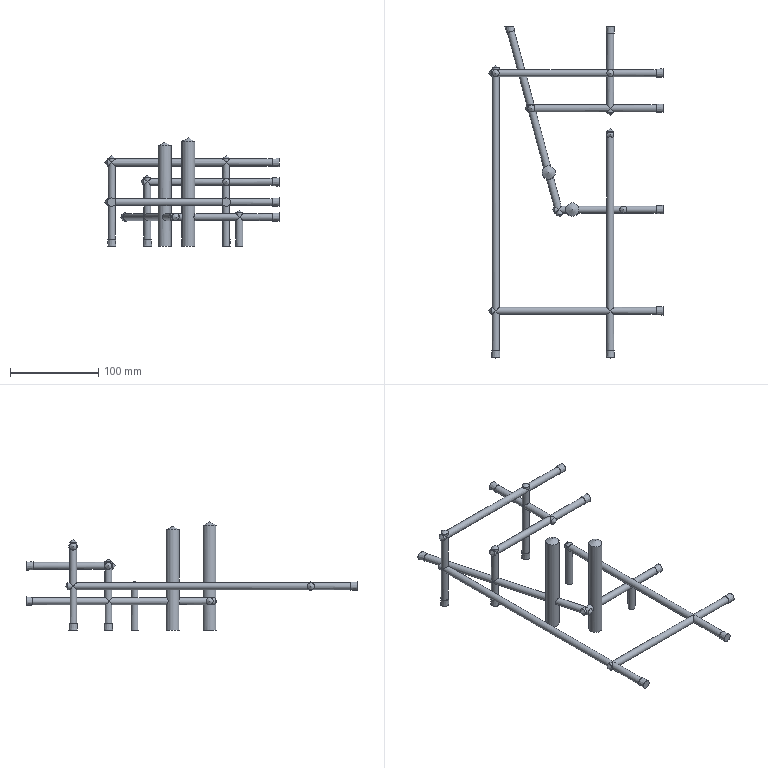Part | STEP file | 车灯-后视镜_id442_x_t | 1 solid | 92 faces | box 197.778 x 377 x 123 mm | volume 135916 mm3 | cylinder 40 | cone 26 | plane 26 | commonest cylinder face diameters 8 x38 15 x2